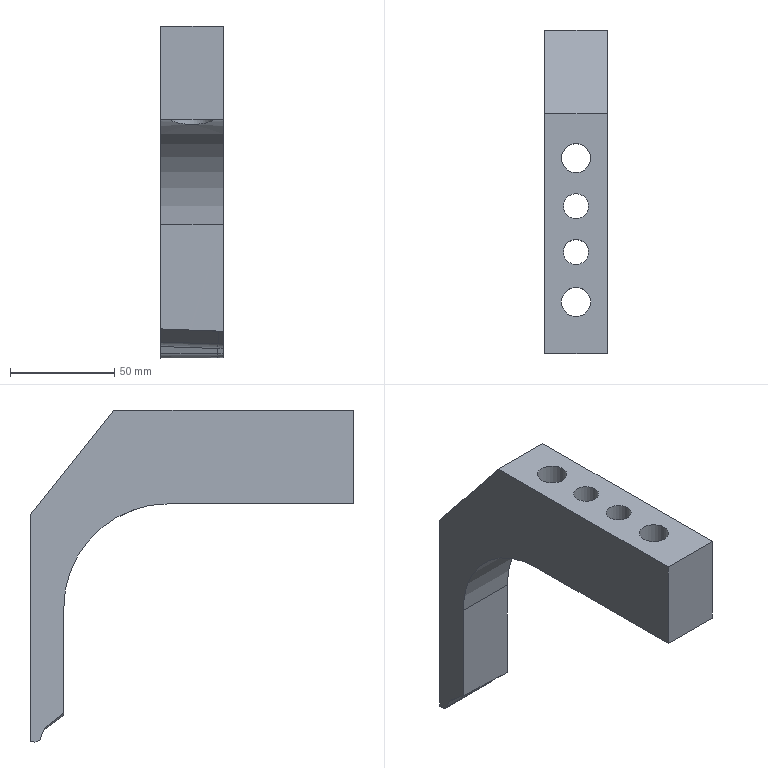Part | NX | features solid 2 | 1 solid | 28 faces | box 30 x 155 x 159.21 mm | volume 216556 mm3 | spline 11 | plane 10 | cylinder 7 | commonest cylinder face diameters 12 x2 14 x2 20 x2 100 x1
STEP:
#1=CARTESIAN_POINT('',(219.476,458.354,-45.808));
#2=VERTEX_POINT('',#1);
#3=CARTESIAN_POINT('',(218.52,458.345,-45.765));
#4=VERTEX_POINT('',#3);
#5=CARTESIAN_POINT('',(219.476,458.35,-45.805));
#6=CARTESIAN_POINT('',(219.157,458.35,-45.791));
#7=CARTESIAN_POINT('',(218.838,458.35,-45.776));
#8=CARTESIAN_POINT('',(218.52,458.35,-45.762));
#9=B_SPLINE_CURVE_WITH_KNOTS('',3,(#5,#6,#7,#8),.UNSPECIFIED.,.F.,.F.,(4,4),(0.,1.),.UNSPECIFIED.);
#10=EDGE_CURVE('',#2,#4,#9,.T.);
#11=ORIENTED_EDGE('',*,*,#10,.F.);
#12=CARTESIAN_POINT('',(235.,458.35,-46.398));
#13=VERTEX_POINT('',#12);
#14=CARTESIAN_POINT('',(219.476,458.35,-45.805));
#15=CARTESIAN_POINT('',(224.651,458.35,-46.003));
#16=CARTESIAN_POINT('',(229.825,458.35,-46.201));
#17=CARTESIAN_POINT('',(235.,458.35,-46.398));
#18=B_SPLINE_CURVE_WITH_KNOTS('',3,(#14,#15,#16,#17),.UNSPECIFIED.,.F.,.F.,(4,4),(0.,0.01554),.UNSPECIFIED.);
#19=EDGE_CURVE('',#2,#13,#18,.T.);
#20=ORIENTED_EDGE('',*,*,#19,.T.);
#21=CARTESIAN_POINT('',(235.,458.35,5.));
#22=VERTEX_POINT('',#21);
#23=CARTESIAN_POINT('',(235.,458.35,-200.));
#24=DIRECTION('',(0.,0.,1.));
#25=VECTOR('',#24,1000.);
#26=LINE('',#23,#25);
#27=EDGE_CURVE('',#13,#22,#26,.T.);
#28=ORIENTED_EDGE('',*,*,#27,.T.);
#29=CARTESIAN_POINT('',(205.,458.35,5.));
#30=VERTEX_POINT('',#29);
#31=CARTESIAN_POINT('',(205.,458.35,5.));
#32=DIRECTION('',(1.,0.,0.));
#33=VECTOR('',#32,1000.);
#34=LINE('',#31,#33);
#35=EDGE_CURVE('',#22,#30,#34,.F.);
#36=ORIENTED_EDGE('',*,*,#35,.T.);
#37=CARTESIAN_POINT('',(205.,458.35,-45.251));
#38=VERTEX_POINT('',#37);
#39=CARTESIAN_POINT('',(205.,458.35,-200.));
#40=DIRECTION('',(0.,0.,1.));
#41=VECTOR('',#40,1000.);
#42=LINE('',#39,#41);
#43=EDGE_CURVE('',#38,#30,#42,.T.);
#44=ORIENTED_EDGE('',*,*,#43,.F.);
#45=CARTESIAN_POINT('',(218.519,458.35,-45.768));
#46=CARTESIAN_POINT('',(214.013,458.35,-45.596));
#47=CARTESIAN_POINT('',(209.506,458.35,-45.423));
#48=CARTESIAN_POINT('',(205.,458.35,-45.251));
#49=B_SPLINE_CURVE_WITH_KNOTS('',3,(#45,#46,#47,#48),.UNSPECIFIED.,.F.,.F.,(4,4),(0.01485,0.02838),.UNSPECIFIED.);
#50=EDGE_CURVE('',#4,#38,#49,.T.);
#51=ORIENTED_EDGE('',*,*,#50,.F.);
#52=EDGE_LOOP('',(#11,#20,#28,#36,#44,#51));
#53=FACE_BOUND('',#52,.T.);
#54=CARTESIAN_POINT('',(220.,458.35,77.5));
#55=DIRECTION('',(0.,1.,0.));
#56=DIRECTION('',(0.,0.,1.));
#57=AXIS2_PLACEMENT_3D('',#54,#55,#56);
#58=PLANE('',#57);
#59=ADVANCED_FACE('',(#53),#58,.F.);
#60=CARTESIAN_POINT('',(235.,474.35,-58.987));
#61=VERTEX_POINT('',#60);
#62=CARTESIAN_POINT('',(235.,472.243,-59.028));
#63=VERTEX_POINT('',#62);
#64=CARTESIAN_POINT('',(235.,474.35,-58.987));
#65=CARTESIAN_POINT('',(235.,473.648,-59.));
#66=CARTESIAN_POINT('',(235.,472.945,-59.014));
#67=CARTESIAN_POINT('',(235.,472.243,-59.028));
#68=B_SPLINE_CURVE_WITH_KNOTS('',3,(#64,#65,#66,#67),.UNSPECIFIED.,.F.,.F.,(4,4),(0.,0.002107),.UNSPECIFIED.);
#69=EDGE_CURVE('',#61,#63,#68,.T.);
#70=ORIENTED_EDGE('',*,*,#69,.F.);
#71=CARTESIAN_POINT('',(235.,474.35,50.));
#72=VERTEX_POINT('',#71);
#73=CARTESIAN_POINT('',(235.,474.35,-200.));
#74=DIRECTION('',(0.,0.,-1.));
#75=VECTOR('',#74,1000.);
#76=LINE('',#73,#75);
#77=EDGE_CURVE('',#72,#61,#76,.T.);
#78=ORIENTED_EDGE('',*,*,#77,.F.);
#79=CARTESIAN_POINT('',(235.,434.35,100.));
#80=VERTEX_POINT('',#79);
#81=CARTESIAN_POINT('',(235.,548.165,-42.268));
#82=DIRECTION('',(0.,0.6247,-0.7809));
#83=VECTOR('',#82,1000.);
#84=LINE('',#81,#83);
#85=EDGE_CURVE('',#72,#80,#84,.F.);
#86=ORIENTED_EDGE('',*,*,#85,.T.);
#87=CARTESIAN_POINT('',(235.,319.35,100.));
#88=VERTEX_POINT('',#87);
#89=CARTESIAN_POINT('',(235.,351.,100.));
#90=DIRECTION('',(0.,1.,0.));
#91=VECTOR('',#90,1000.);
#92=LINE('',#89,#91);
#93=EDGE_CURVE('',#88,#80,#92,.T.);
#94=ORIENTED_EDGE('',*,*,#93,.F.);
#95=CARTESIAN_POINT('',(235.,319.35,55.));
#96=VERTEX_POINT('',#95);
#97=CARTESIAN_POINT('',(235.,319.35,-200.));
#98=DIRECTION('',(0.,0.,1.));
#99=VECTOR('',#98,1000.);
#100=LINE('',#97,#99);
#101=EDGE_CURVE('',#96,#88,#100,.T.);
#102=ORIENTED_EDGE('',*,*,#101,.F.);
#103=CARTESIAN_POINT('',(235.,408.35,55.));
#104=VERTEX_POINT('',#103);
#105=CARTESIAN_POINT('',(235.,351.,55.));
#106=DIRECTION('',(0.,1.,0.));
#107=VECTOR('',#106,1000.);
#108=LINE('',#105,#107);
#109=EDGE_CURVE('',#96,#104,#108,.T.);
#110=ORIENTED_EDGE('',*,*,#109,.T.);
#111=CARTESIAN_POINT('',(235.,408.35,5.));
#112=DIRECTION('',(1.,0.,0.));
#113=DIRECTION('',(0.,0.,-1.));
#114=AXIS2_PLACEMENT_3D('',#111,#112,#113);
#115=CIRCLE('',#114,50.);
#116=EDGE_CURVE('',#104,#22,#115,.F.);
#117=ORIENTED_EDGE('',*,*,#116,.T.);
#118=ORIENTED_EDGE('',*,*,#27,.F.);
#119=CARTESIAN_POINT('',(235.,458.502,-46.511));
#120=VERTEX_POINT('',#119);
#121=CARTESIAN_POINT('',(235.,458.502,-46.511));
#122=CARTESIAN_POINT('',(235.,458.451,-46.474));
#123=CARTESIAN_POINT('',(235.,458.4,-46.437));
#124=CARTESIAN_POINT('',(235.,458.35,-46.398));
#125=B_SPLINE_CURVE_WITH_KNOTS('',3,(#121,#122,#123,#124),.UNSPECIFIED.,.F.,.F.,(4,4),(0.,0.0001883),.UNSPECIFIED.);
#126=EDGE_CURVE('',#120,#13,#125,.T.);
#127=ORIENTED_EDGE('',*,*,#126,.F.);
#128=CARTESIAN_POINT('',(235.,466.758,-52.527));
#129=VERTEX_POINT('',#128);
#130=CARTESIAN_POINT('',(235.,458.502,-46.512));
#131=CARTESIAN_POINT('',(235.,461.253,-48.519));
#132=CARTESIAN_POINT('',(235.,464.006,-50.524));
#133=CARTESIAN_POINT('',(235.,466.76,-52.528));
#134=B_SPLINE_CURVE_WITH_KNOTS('',3,(#130,#131,#132,#133),.UNSPECIFIED.,.F.,.F.,(4,4),(0.00008632,0.0103),.UNSPECIFIED.);
#135=EDGE_CURVE('',#120,#129,#134,.T.);
#136=ORIENTED_EDGE('',*,*,#135,.T.);
#137=CARTESIAN_POINT('',(235.,468.481,-54.772));
#138=VERTEX_POINT('',#137);
#139=CARTESIAN_POINT('',(235.,468.482,-54.771));
#140=CARTESIAN_POINT('',(235.,468.136,-53.875));
#141=CARTESIAN_POINT('',(235.,467.534,-53.091));
#142=CARTESIAN_POINT('',(235.,466.757,-52.526));
#143=B_SPLINE_CURVE_WITH_KNOTS('',3,(#139,#140,#141,#142),.UNSPECIFIED.,.F.,.F.,(4,4),(0.,0.002874),.UNSPECIFIED.);
#144=EDGE_CURVE('',#138,#129,#143,.T.);
#145=ORIENTED_EDGE('',*,*,#144,.F.);
#146=CARTESIAN_POINT('',(235.,469.383,-57.108));
#147=VERTEX_POINT('',#146);
#148=CARTESIAN_POINT('',(235.,469.381,-57.106));
#149=CARTESIAN_POINT('',(235.,469.08,-56.328));
#150=CARTESIAN_POINT('',(235.,468.78,-55.551));
#151=CARTESIAN_POINT('',(235.,468.48,-54.774));
#152=B_SPLINE_CURVE_WITH_KNOTS('',3,(#148,#149,#150,#151),.UNSPECIFIED.,.F.,.F.,(4,4),(0.00004866,0.002549),.UNSPECIFIED.);
#153=EDGE_CURVE('',#147,#138,#152,.T.);
#154=ORIENTED_EDGE('',*,*,#153,.F.);
#155=CARTESIAN_POINT('',(235.,472.243,-59.028));
#156=CARTESIAN_POINT('',(235.,471.011,-59.052));
#157=CARTESIAN_POINT('',(235.,469.83,-58.259));
#158=CARTESIAN_POINT('',(235.,469.386,-57.11));
#159=B_SPLINE_CURVE_WITH_KNOTS('',3,(#155,#156,#157,#158),.UNSPECIFIED.,.F.,.F.,(4,4),(0.,0.003644),.UNSPECIFIED.);
#160=EDGE_CURVE('',#63,#147,#159,.T.);
#161=ORIENTED_EDGE('',*,*,#160,.F.);
#162=EDGE_LOOP('',(#70,#78,#86,#94,#102,#110,#117,#118,#127,#136,#145,#154,#161));
#163=FACE_BOUND('',#162,.T.);
#164=CARTESIAN_POINT('',(235.,351.,-200.));
#165=DIRECTION('',(1.,0.,0.));
#166=DIRECTION('',(0.,0.,-1.));
#167=AXIS2_PLACEMENT_3D('',#164,#165,#166);
#168=PLANE('',#167);
#169=ADVANCED_FACE('',(#163),#168,.T.);
#170=CARTESIAN_POINT('',(205.,474.35,50.));
#171=VERTEX_POINT('',#170);
#172=CARTESIAN_POINT('',(205.,474.35,-59.17));
#173=VERTEX_POINT('',#172);
#174=CARTESIAN_POINT('',(205.,474.35,-200.));
#175=DIRECTION('',(0.,0.,-1.));
#176=VECTOR('',#175,1000.);
#177=LINE('',#174,#176);
#178=EDGE_CURVE('',#171,#173,#177,.T.);
#179=ORIENTED_EDGE('',*,*,#178,.T.);
#180=CARTESIAN_POINT('',(205.,472.244,-59.21));
#181=VERTEX_POINT('',#180);
#182=CARTESIAN_POINT('',(205.,474.35,-59.17));
#183=CARTESIAN_POINT('',(205.,473.646,-59.183));
#184=CARTESIAN_POINT('',(205.,472.942,-59.197));
#185=CARTESIAN_POINT('',(205.,472.239,-59.21));
#186=B_SPLINE_CURVE_WITH_KNOTS('',3,(#182,#183,#184,#185),.UNSPECIFIED.,.F.,.F.,(4,4),(0.,0.002112),.UNSPECIFIED.);
#187=EDGE_CURVE('',#173,#181,#186,.T.);
#188=ORIENTED_EDGE('',*,*,#187,.T.);
#189=CARTESIAN_POINT('',(205.,469.389,-57.288));
#190=VERTEX_POINT('',#189);
#191=CARTESIAN_POINT('',(205.,472.245,-59.21));
#192=CARTESIAN_POINT('',(205.,471.012,-59.232));
#193=CARTESIAN_POINT('',(205.,469.832,-58.438));
#194=CARTESIAN_POINT('',(205.,469.389,-57.288));
#195=B_SPLINE_CURVE_WITH_KNOTS('',3,(#191,#192,#193,#194),.UNSPECIFIED.,.F.,.F.,(4,4),(0.,0.003644),.UNSPECIFIED.);
#196=EDGE_CURVE('',#181,#190,#195,.T.);
#197=ORIENTED_EDGE('',*,*,#196,.T.);
#198=CARTESIAN_POINT('',(205.,468.012,-53.711));
#199=VERTEX_POINT('',#198);
#200=CARTESIAN_POINT('',(205.,469.389,-57.288));
#201=CARTESIAN_POINT('',(205.,468.93,-56.096));
#202=CARTESIAN_POINT('',(205.,468.471,-54.903));
#203=CARTESIAN_POINT('',(205.,468.012,-53.711));
#204=B_SPLINE_CURVE_WITH_KNOTS('',3,(#200,#201,#202,#203),.UNSPECIFIED.,.F.,.F.,(4,4),(0.0000259,0.003859),.UNSPECIFIED.);
#205=EDGE_CURVE('',#190,#199,#204,.T.);
#206=ORIENTED_EDGE('',*,*,#205,.T.);
#207=CARTESIAN_POINT('',(205.,466.425,-51.567));
#208=VERTEX_POINT('',#207);
#209=CARTESIAN_POINT('',(205.,468.012,-53.711));
#210=CARTESIAN_POINT('',(205.,467.688,-52.868));
#211=CARTESIAN_POINT('',(205.,467.136,-52.123));
#212=CARTESIAN_POINT('',(205.,466.425,-51.567));
#213=B_SPLINE_CURVE_WITH_KNOTS('',3,(#209,#210,#211,#212),.UNSPECIFIED.,.F.,.F.,(4,4),(0.,0.002703),.UNSPECIFIED.);
#214=EDGE_CURVE('',#199,#208,#213,.T.);
#215=ORIENTED_EDGE('',*,*,#214,.T.);
#216=CARTESIAN_POINT('',(205.,458.35,-45.251));
#217=CARTESIAN_POINT('',(205.,461.041,-47.356));
#218=CARTESIAN_POINT('',(205.,463.733,-49.461));
#219=CARTESIAN_POINT('',(205.,466.425,-51.567));
#220=B_SPLINE_CURVE_WITH_KNOTS('',3,(#216,#217,#218,#219),.UNSPECIFIED.,.F.,.F.,(4,4),(0.0006093,0.01086),.UNSPECIFIED.);
#221=EDGE_CURVE('',#38,#208,#220,.T.);
#222=ORIENTED_EDGE('',*,*,#221,.F.);
#223=ORIENTED_EDGE('',*,*,#43,.T.);
#224=CARTESIAN_POINT('',(205.,408.35,55.));
#225=VERTEX_POINT('',#224);
#226=CARTESIAN_POINT('',(205.,408.35,5.));
#227=DIRECTION('',(1.,0.,0.));
#228=DIRECTION('',(0.,0.,-1.));
#229=AXIS2_PLACEMENT_3D('',#226,#227,#228);
#230=CIRCLE('',#229,50.);
#231=EDGE_CURVE('',#30,#225,#230,.T.);
#232=ORIENTED_EDGE('',*,*,#231,.T.);
#233=CARTESIAN_POINT('',(205.,319.35,55.));
#234=VERTEX_POINT('',#233);
#235=CARTESIAN_POINT('',(205.,431.,55.));
#236=DIRECTION('',(0.,1.,0.));
#237=VECTOR('',#236,1000.);
#238=LINE('',#235,#237);
#239=EDGE_CURVE('',#225,#234,#238,.F.);
#240=ORIENTED_EDGE('',*,*,#239,.T.);
#241=CARTESIAN_POINT('',(205.,319.35,100.));
#242=VERTEX_POINT('',#241);
#243=CARTESIAN_POINT('',(205.,319.35,-200.));
#244=DIRECTION('',(0.,0.,1.));
#245=VECTOR('',#244,1000.);
#246=LINE('',#243,#245);
#247=EDGE_CURVE('',#234,#242,#246,.T.);
#248=ORIENTED_EDGE('',*,*,#247,.T.);
#249=CARTESIAN_POINT('',(205.,434.35,100.));
#250=VERTEX_POINT('',#249);
#251=CARTESIAN_POINT('',(205.,351.,100.));
#252=DIRECTION('',(0.,1.,0.));
#253=VECTOR('',#252,1000.);
#254=LINE('',#251,#253);
#255=EDGE_CURVE('',#242,#250,#254,.T.);
#256=ORIENTED_EDGE('',*,*,#255,.T.);
#257=CARTESIAN_POINT('',(205.,434.35,100.));
#258=DIRECTION('',(0.,-0.6247,0.7809));
#259=VECTOR('',#258,1000.);
#260=LINE('',#257,#259);
#261=EDGE_CURVE('',#250,#171,#260,.F.);
#262=ORIENTED_EDGE('',*,*,#261,.T.);
#263=EDGE_LOOP('',(#179,#188,#197,#206,#215,#222,#223,#232,#240,#248,#256,#262));
#264=FACE_BOUND('',#263,.T.);
#265=CARTESIAN_POINT('',(205.,351.,-200.));
#266=DIRECTION('',(1.,0.,0.));
#267=DIRECTION('',(0.,0.,-1.));
#268=AXIS2_PLACEMENT_3D('',#265,#266,#267);
#269=PLANE('',#268);
#270=ADVANCED_FACE('',(#264),#269,.F.);
#271=ORIENTED_EDGE('',*,*,#247,.F.);
#272=CARTESIAN_POINT('',(235.,319.35,55.));
#273=DIRECTION('',(-1.,0.,0.));
#274=VECTOR('',#273,1000.);
#275=LINE('',#272,#274);
#276=EDGE_CURVE('',#96,#234,#275,.T.);
#277=ORIENTED_EDGE('',*,*,#276,.F.);
#278=ORIENTED_EDGE('',*,*,#101,.T.);
#279=CARTESIAN_POINT('',(275.,319.35,100.));
#280=DIRECTION('',(-1.,0.,0.));
#281=VECTOR('',#280,1000.);
#282=LINE('',#279,#281);
#283=EDGE_CURVE('',#88,#242,#282,.T.);
#284=ORIENTED_EDGE('',*,*,#283,.T.);
#285=EDGE_LOOP('',(#271,#277,#278,#284));
#286=FACE_BOUND('',#285,.T.);
#287=CARTESIAN_POINT('',(275.,319.35,75.));
#288=DIRECTION('',(0.,1.,0.));
#289=DIRECTION('',(0.,0.,1.));
#290=AXIS2_PLACEMENT_3D('',#287,#288,#289);
#291=PLANE('',#290);
#292=ADVANCED_FACE('',(#286),#291,.F.);
#293=CARTESIAN_POINT('',(214.,368.,100.));
#294=VERTEX_POINT('',#293);
#295=CARTESIAN_POINT('',(220.,368.,100.));
#296=DIRECTION('',(0.,0.,-1.));
#297=DIRECTION('',(-1.,0.,0.));
#298=AXIS2_PLACEMENT_3D('',#295,#296,#297);
#299=CIRCLE('',#298,6.);
#300=EDGE_CURVE('',#294,#294,#299,.T.);
#301=ORIENTED_EDGE('',*,*,#300,.T.);
#302=EDGE_LOOP('',(#301));
#303=FACE_BOUND('',#302,.T.);
#304=CARTESIAN_POINT('',(214.,390.,100.));
#305=VERTEX_POINT('',#304);
#306=CARTESIAN_POINT('',(220.,390.,100.));
#307=DIRECTION('',(0.,0.,-1.));
#308=DIRECTION('',(-1.,0.,0.));
#309=AXIS2_PLACEMENT_3D('',#306,#307,#308);
#310=CIRCLE('',#309,6.);
#311=EDGE_CURVE('',#305,#305,#310,.T.);
#312=ORIENTED_EDGE('',*,*,#311,.T.);
#313=EDGE_LOOP('',(#312));
#314=FACE_BOUND('',#313,.T.);
#315=CARTESIAN_POINT('',(213.,344.,100.));
#316=VERTEX_POINT('',#315);
#317=CARTESIAN_POINT('',(220.,344.,100.));
#318=DIRECTION('',(0.,0.,-1.));
#319=DIRECTION('',(-1.,0.,0.));
#320=AXIS2_PLACEMENT_3D('',#317,#318,#319);
#321=CIRCLE('',#320,7.);
#322=EDGE_CURVE('',#316,#316,#321,.T.);
#323=ORIENTED_EDGE('',*,*,#322,.T.);
#324=EDGE_LOOP('',(#323));
#325=FACE_BOUND('',#324,.T.);
#326=CARTESIAN_POINT('',(213.,413.,100.));
#327=VERTEX_POINT('',#326);
#328=CARTESIAN_POINT('',(220.,413.,100.));
#329=DIRECTION('',(0.,0.,-1.));
#330=DIRECTION('',(-1.,0.,0.));
#331=AXIS2_PLACEMENT_3D('',#328,#329,#330);
#332=CIRCLE('',#331,7.);
#333=EDGE_CURVE('',#327,#327,#332,.T.);
#334=ORIENTED_EDGE('',*,*,#333,.T.);
#335=EDGE_LOOP('',(#334));
#336=FACE_BOUND('',#335,.T.);
#337=ORIENTED_EDGE('',*,*,#93,.T.);
#338=CARTESIAN_POINT('',(160.,434.35,100.));
#339=DIRECTION('',(-1.,0.,0.));
#340=VECTOR('',#339,1000.);
#341=LINE('',#338,#340);
#342=EDGE_CURVE('',#80,#250,#341,.T.);
#343=ORIENTED_EDGE('',*,*,#342,.T.);
#344=ORIENTED_EDGE('',*,*,#255,.F.);
#345=ORIENTED_EDGE('',*,*,#283,.F.);
#346=EDGE_LOOP('',(#337,#343,#344,#345));
#347=FACE_BOUND('',#346,.T.);
#348=CARTESIAN_POINT('',(160.,351.,100.));
#349=DIRECTION('',(0.,0.,-1.));
#350=DIRECTION('',(-1.,0.,0.));
#351=AXIS2_PLACEMENT_3D('',#348,#349,#350);
#352=PLANE('',#351);
#353=ADVANCED_FACE('',(#303,#314,#325,#336,#347),#352,.F.);
#354=CARTESIAN_POINT('',(227.,413.,75.));
#355=VERTEX_POINT('',#354);
#356=CARTESIAN_POINT('',(220.,413.,75.));
#357=DIRECTION('',(0.,0.,1.));
#358=DIRECTION('',(1.,0.,0.));
#359=AXIS2_PLACEMENT_3D('',#356,#357,#358);
#360=CIRCLE('',#359,7.);
#361=EDGE_CURVE('',#355,#355,#360,.T.);
#362=ORIENTED_EDGE('',*,*,#361,.F.);
#363=EDGE_LOOP('',(#362));
#364=FACE_BOUND('',#363,.T.);
#365=ORIENTED_EDGE('',*,*,#333,.F.);
#366=EDGE_LOOP('',(#365));
#367=FACE_BOUND('',#366,.T.);
#368=CARTESIAN_POINT('',(220.,413.,75.));
#369=DIRECTION('',(0.,0.,1.));
#370=DIRECTION('',(-1.,0.,0.));
#371=AXIS2_PLACEMENT_3D('',#368,#369,#370);
#372=CYLINDRICAL_SURFACE('',#371,7.);
#373=ADVANCED_FACE('',(#364,#367),#372,.F.);
#374=ORIENTED_EDGE('',*,*,#361,.T.);
#375=EDGE_LOOP('',(#374));
#376=FACE_BOUND('',#375,.T.);
#377=CARTESIAN_POINT('',(230.,413.,75.));
#378=VERTEX_POINT('',#377);
#379=CARTESIAN_POINT('',(220.,413.,75.));
#380=DIRECTION('',(0.,0.,-1.));
#381=DIRECTION('',(1.,0.,0.));
#382=AXIS2_PLACEMENT_3D('',#379,#380,#381);
#383=CIRCLE('',#382,10.);
#384=EDGE_CURVE('',#378,#378,#383,.T.);
#385=ORIENTED_EDGE('',*,*,#384,.T.);
#386=EDGE_LOOP('',(#385));
#387=FACE_BOUND('',#386,.T.);
#388=CARTESIAN_POINT('',(220.,413.,75.));
#389=DIRECTION('',(0.,0.,1.));
#390=DIRECTION('',(-1.,0.,0.));
#391=AXIS2_PLACEMENT_3D('',#388,#389,#390);
#392=PLANE('',#391);
#393=ADVANCED_FACE('',(#376,#387),#392,.F.);
#394=CARTESIAN_POINT('',(228.853,408.35,55.));
#395=VERTEX_POINT('',#394);
#396=CARTESIAN_POINT('',(211.147,408.35,55.));
#397=VERTEX_POINT('',#396);
#398=CARTESIAN_POINT('',(220.,413.,55.));
#399=DIRECTION('',(0.,0.,1.));
#400=DIRECTION('',(1.,0.,0.));
#401=AXIS2_PLACEMENT_3D('',#398,#399,#400);
#402=CIRCLE('',#401,10.);
#403=EDGE_CURVE('',#395,#397,#402,.F.);
#404=ORIENTED_EDGE('',*,*,#403,.T.);
#405=CARTESIAN_POINT('',(211.147,408.35,55.));
#406=CARTESIAN_POINT('',(210.338,409.891,55.));
#407=CARTESIAN_POINT('',(209.557,413.344,54.846));
#408=CARTESIAN_POINT('',(211.077,418.422,54.048));
#409=CARTESIAN_POINT('',(214.831,422.077,53.101));
#410=CARTESIAN_POINT('',(219.999,423.459,52.658));
#411=CARTESIAN_POINT('',(225.153,422.088,53.099));
#412=CARTESIAN_POINT('',(228.929,418.412,54.049));
#413=CARTESIAN_POINT('',(230.441,413.366,54.844));
#414=CARTESIAN_POINT('',(229.663,409.891,55.));
#415=CARTESIAN_POINT('',(228.853,408.35,55.));
#416=B_SPLINE_CURVE_WITH_KNOTS('',3,(#405,#406,#407,#408,#409,#410,#411,#412,#413,#414,#415),.UNSPECIFIED.,.F.,.F.,(4,1,1,1,1,1,1,1,4),(0.,0.005148,0.0103,0.01544,0.02059,0.02574,0.03089,0.03603,0.04118),.UNSPECIFIED.);
#417=EDGE_CURVE('',#397,#395,#416,.T.);
#418=ORIENTED_EDGE('',*,*,#417,.T.);
#419=EDGE_LOOP('',(#404,#418));
#420=FACE_BOUND('',#419,.T.);
#421=ORIENTED_EDGE('',*,*,#384,.F.);
#422=EDGE_LOOP('',(#421));
#423=FACE_BOUND('',#422,.T.);
#424=CARTESIAN_POINT('',(220.,413.,75.));
#425=DIRECTION('',(0.,0.,-1.));
#426=DIRECTION('',(1.,0.,0.));
#427=AXIS2_PLACEMENT_3D('',#424,#425,#426);
#428=CYLINDRICAL_SURFACE('',#427,10.);
#429=ADVANCED_FACE('',(#420,#423),#428,.F.);
#430=CARTESIAN_POINT('',(227.,344.,75.));
#431=VERTEX_POINT('',#430);
#432=CARTESIAN_POINT('',(220.,344.,75.));
#433=DIRECTION('',(0.,0.,1.));
#434=DIRECTION('',(1.,0.,0.));
#435=AXIS2_PLACEMENT_3D('',#432,#433,#434);
#436=CIRCLE('',#435,7.);
#437=EDGE_CURVE('',#431,#431,#436,.T.);
#438=ORIENTED_EDGE('',*,*,#437,.F.);
#439=EDGE_LOOP('',(#438));
#440=FACE_BOUND('',#439,.T.);
#441=ORIENTED_EDGE('',*,*,#322,.F.);
#442=EDGE_LOOP('',(#441));
#443=FACE_BOUND('',#442,.T.);
#444=CARTESIAN_POINT('',(220.,344.,75.));
#445=DIRECTION('',(0.,0.,1.));
#446=DIRECTION('',(-1.,0.,0.));
#447=AXIS2_PLACEMENT_3D('',#444,#445,#446);
#448=CYLINDRICAL_SURFACE('',#447,7.);
#449=ADVANCED_FACE('',(#440,#443),#448,.F.);
#450=CARTESIAN_POINT('',(230.,344.,55.));
#451=VERTEX_POINT('',#450);
#452=CARTESIAN_POINT('',(220.,344.,55.));
#453=DIRECTION('',(0.,0.,1.));
#454=DIRECTION('',(1.,0.,0.));
#455=AXIS2_PLACEMENT_3D('',#452,#453,#454);
#456=CIRCLE('',#455,10.);
#457=EDGE_CURVE('',#451,#451,#456,.F.);
#458=ORIENTED_EDGE('',*,*,#457,.T.);
#459=EDGE_LOOP('',(#458));
#460=FACE_BOUND('',#459,.T.);
#461=CARTESIAN_POINT('',(230.,344.,75.));
#462=VERTEX_POINT('',#461);
#463=CARTESIAN_POINT('',(220.,344.,75.));
#464=DIRECTION('',(0.,0.,-1.));
#465=DIRECTION('',(1.,0.,0.));
#466=AXIS2_PLACEMENT_3D('',#463,#464,#465);
#467=CIRCLE('',#466,10.);
#468=EDGE_CURVE('',#462,#462,#467,.T.);
#469=ORIENTED_EDGE('',*,*,#468,.F.);
#470=EDGE_LOOP('',(#469));
#471=FACE_BOUND('',#470,.T.);
#472=CARTESIAN_POINT('',(220.,344.,75.));
#473=DIRECTION('',(0.,0.,-1.));
#474=DIRECTION('',(1.,0.,0.));
#475=AXIS2_PLACEMENT_3D('',#472,#473,#474);
#476=CYLINDRICAL_SURFACE('',#475,10.);
#477=ADVANCED_FACE('',(#460,#471),#476,.F.);
#478=ORIENTED_EDGE('',*,*,#437,.T.);
#479=EDGE_LOOP('',(#478));
#480=FACE_BOUND('',#479,.T.);
#481=ORIENTED_EDGE('',*,*,#468,.T.);
#482=EDGE_LOOP('',(#481));
#483=FACE_BOUND('',#482,.T.);
#484=CARTESIAN_POINT('',(220.,344.,75.));
#485=DIRECTION('',(0.,0.,1.));
#486=DIRECTION('',(-1.,0.,0.));
#487=AXIS2_PLACEMENT_3D('',#484,#485,#486);
#488=PLANE('',#487);
#489=ADVANCED_FACE('',(#480,#483),#488,.F.);
#490=CARTESIAN_POINT('',(214.,368.,55.));
#491=VERTEX_POINT('',#490);
#492=CARTESIAN_POINT('',(220.,368.,55.));
#493=DIRECTION('',(0.,0.,-1.));
#494=DIRECTION('',(-1.,0.,0.));
#495=AXIS2_PLACEMENT_3D('',#492,#493,#494);
#496=CIRCLE('',#495,6.);
#497=EDGE_CURVE('',#491,#491,#496,.T.);
#498=ORIENTED_EDGE('',*,*,#497,.F.);
#499=EDGE_LOOP('',(#498));
#500=FACE_BOUND('',#499,.T.);
#501=CARTESIAN_POINT('',(214.,390.,55.));
#502=VERTEX_POINT('',#501);
#503=CARTESIAN_POINT('',(220.,390.,55.));
#504=DIRECTION('',(0.,0.,-1.));
#505=DIRECTION('',(-1.,0.,0.));
#506=AXIS2_PLACEMENT_3D('',#503,#504,#505);
#507=CIRCLE('',#506,6.);
#508=EDGE_CURVE('',#502,#502,#507,.T.);
#509=ORIENTED_EDGE('',*,*,#508,.F.);
#510=EDGE_LOOP('',(#509));
#511=FACE_BOUND('',#510,.T.);
#512=ORIENTED_EDGE('',*,*,#457,.F.);
#513=EDGE_LOOP('',(#512));
#514=FACE_BOUND('',#513,.T.);
#515=ORIENTED_EDGE('',*,*,#239,.F.);
#516=CARTESIAN_POINT('',(235.,408.35,55.));
#517=DIRECTION('',(1.,0.,0.));
#518=VECTOR('',#517,1000.);
#519=LINE('',#516,#518);
#520=EDGE_CURVE('',#225,#397,#519,.T.);
#521=ORIENTED_EDGE('',*,*,#520,.T.);
#522=ORIENTED_EDGE('',*,*,#403,.F.);
#523=CARTESIAN_POINT('',(235.,408.35,55.));
#524=DIRECTION('',(1.,0.,0.));
#525=VECTOR('',#524,1000.);
#526=LINE('',#523,#525);
#527=EDGE_CURVE('',#395,#104,#526,.T.);
#528=ORIENTED_EDGE('',*,*,#527,.T.);
#529=ORIENTED_EDGE('',*,*,#109,.F.);
#530=ORIENTED_EDGE('',*,*,#276,.T.);
#531=EDGE_LOOP('',(#515,#521,#522,#528,#529,#530));
#532=FACE_BOUND('',#531,.T.);
#533=CARTESIAN_POINT('',(235.,431.,55.));
#534=DIRECTION('',(0.,0.,1.));
#535=DIRECTION('',(1.,0.,0.));
#536=AXIS2_PLACEMENT_3D('',#533,#534,#535);
#537=PLANE('',#536);
#538=ADVANCED_FACE('',(#500,#511,#514,#532),#537,.F.);
#539=ORIENTED_EDGE('',*,*,#311,.F.);
#540=EDGE_LOOP('',(#539));
#541=FACE_BOUND('',#540,.T.);
#542=ORIENTED_EDGE('',*,*,#508,.T.);
#543=EDGE_LOOP('',(#542));
#544=FACE_BOUND('',#543,.T.);
#545=CARTESIAN_POINT('',(220.,390.,105.));
#546=DIRECTION('',(0.,0.,-1.));
#547=DIRECTION('',(-1.,0.,0.));
#548=AXIS2_PLACEMENT_3D('',#545,#546,#547);
#549=CYLINDRICAL_SURFACE('',#548,6.);
#550=ADVANCED_FACE('',(#541,#544),#549,.F.);
#551=ORIENTED_EDGE('',*,*,#300,.F.);
#552=EDGE_LOOP('',(#551));
#553=FACE_BOUND('',#552,.T.);
#554=ORIENTED_EDGE('',*,*,#497,.T.);
#555=EDGE_LOOP('',(#554));
#556=FACE_BOUND('',#555,.T.);
#557=CARTESIAN_POINT('',(220.,368.,105.));
#558=DIRECTION('',(0.,0.,-1.));
#559=DIRECTION('',(-1.,0.,0.));
#560=AXIS2_PLACEMENT_3D('',#557,#558,#559);
#561=CYLINDRICAL_SURFACE('',#560,6.);
#562=ADVANCED_FACE('',(#553,#556),#561,.F.);
#563=ORIENTED_EDGE('',*,*,#77,.T.);
#564=CARTESIAN_POINT('',(232.114,474.35,-59.018));
#565=VERTEX_POINT('',#564);
#566=CARTESIAN_POINT('',(235.,474.35,-58.987));
#567=CARTESIAN_POINT('',(234.038,474.35,-58.997));
#568=CARTESIAN_POINT('',(233.076,474.35,-59.008));
#569=CARTESIAN_POINT('',(232.114,474.35,-59.018));
#570=B_SPLINE_CURVE_WITH_KNOTS('',3,(#566,#567,#568,#569),.UNSPECIFIED.,.F.,.F.,(4,4),(0.,0.002886),.UNSPECIFIED.);
#571=EDGE_CURVE('',#61,#565,#570,.T.);
#572=ORIENTED_EDGE('',*,*,#571,.T.);
#573=CARTESIAN_POINT('',(232.114,474.35,-59.018));
#574=CARTESIAN_POINT('',(223.076,474.35,-59.111));
#575=CARTESIAN_POINT('',(214.038,474.35,-59.162));
#576=CARTESIAN_POINT('',(205.,474.35,-59.17));
#577=B_SPLINE_CURVE_WITH_KNOTS('',3,(#573,#574,#575,#576),.UNSPECIFIED.,.F.,.F.,(4,4),(0.00001661,0.02713),.UNSPECIFIED.);
#578=EDGE_CURVE('',#565,#173,#577,.T.);
#579=ORIENTED_EDGE('',*,*,#578,.T.);
#580=ORIENTED_EDGE('',*,*,#178,.F.);
#581=CARTESIAN_POINT('',(220.,474.35,50.));
#582=DIRECTION('',(1.,0.,0.));
#583=VECTOR('',#582,1000.);
#584=LINE('',#581,#583);
#585=EDGE_CURVE('',#171,#72,#584,.T.);
#586=ORIENTED_EDGE('',*,*,#585,.T.);
#587=EDGE_LOOP('',(#563,#572,#579,#580,#586));
#588=FACE_BOUND('',#587,.T.);
#589=CARTESIAN_POINT('',(220.,474.35,77.5));
#590=DIRECTION('',(0.,-1.,0.));
#591=DIRECTION('',(0.,0.,-1.));
#592=AXIS2_PLACEMENT_3D('',#589,#590,#591);
#593=PLANE('',#592);
#594=ADVANCED_FACE('',(#588),#593,.F.);
#595=ORIENTED_EDGE('',*,*,#231,.F.);
#596=ORIENTED_EDGE('',*,*,#35,.F.);
#597=ORIENTED_EDGE('',*,*,#116,.F.);
#598=ORIENTED_EDGE('',*,*,#527,.F.);
#599=ORIENTED_EDGE('',*,*,#417,.F.);
#600=ORIENTED_EDGE('',*,*,#520,.F.);
#601=EDGE_LOOP('',(#595,#596,#597,#598,#599,#600));
#602=FACE_BOUND('',#601,.T.);
#603=CARTESIAN_POINT('',(235.,408.35,5.));
#604=DIRECTION('',(-1.,0.,0.));
#605=DIRECTION('',(0.,0.,1.));
#606=AXIS2_PLACEMENT_3D('',#603,#604,#605);
#607=CYLINDRICAL_SURFACE('',#606,50.);
#608=ADVANCED_FACE('',(#602),#607,.F.);
#609=ORIENTED_EDGE('',*,*,#85,.F.);
#610=ORIENTED_EDGE('',*,*,#585,.F.);
#611=ORIENTED_EDGE('',*,*,#261,.F.);
#612=ORIENTED_EDGE('',*,*,#342,.F.);
#613=EDGE_LOOP('',(#609,#610,#611,#612));
#614=FACE_BOUND('',#613,.T.);
#615=CARTESIAN_POINT('',(160.,434.35,100.));
#616=DIRECTION('',(0.,-0.7809,-0.6247));
#617=DIRECTION('',(0.,0.6247,-0.7809));
#618=AXIS2_PLACEMENT_3D('',#615,#616,#617);
#619=PLANE('',#618);
#620=ADVANCED_FACE('',(#614),#619,.F.);
#621=CARTESIAN_POINT('',(232.133,472.243,-59.059));
#622=VERTEX_POINT('',#621);
#623=CARTESIAN_POINT('',(232.133,472.243,-59.059));
#624=CARTESIAN_POINT('',(223.089,472.244,-59.151));
#625=CARTESIAN_POINT('',(214.045,472.244,-59.202));
#626=CARTESIAN_POINT('',(205.,472.245,-59.21));
#627=B_SPLINE_CURVE_WITH_KNOTS('',3,(#623,#624,#625,#626),.UNSPECIFIED.,.F.,.F.,(4,4),(0.,0.6639),.UNSPECIFIED.);
#628=EDGE_CURVE('',#181,#622,#627,.F.);
#629=ORIENTED_EDGE('',*,*,#628,.T.);
#630=CARTESIAN_POINT('',(232.249,469.383,-57.14));
#631=VERTEX_POINT('',#630);
#632=CARTESIAN_POINT('',(232.249,469.386,-57.139));
#633=CARTESIAN_POINT('',(232.215,469.65,-57.824));
#634=CARTESIAN_POINT('',(232.162,470.634,-58.849));
#635=CARTESIAN_POINT('',(232.137,471.756,-59.068));
#636=CARTESIAN_POINT('',(232.133,472.243,-59.059));
#637=B_SPLINE_CURVE_WITH_KNOTS('',3,(#632,#633,#634,#635,#636),.UNSPECIFIED.,.F.,.F.,(4,1,4),(0.,0.5,1.),.UNSPECIFIED.);
#638=EDGE_CURVE('',#622,#631,#637,.F.);
#639=ORIENTED_EDGE('',*,*,#638,.T.);
#640=CARTESIAN_POINT('',(205.,469.389,-57.288));
#641=CARTESIAN_POINT('',(214.083,469.388,-57.281));
#642=CARTESIAN_POINT('',(223.166,469.387,-57.231));
#643=CARTESIAN_POINT('',(232.249,469.386,-57.139));
#644=B_SPLINE_CURVE_WITH_KNOTS('',3,(#640,#641,#642,#643),.UNSPECIFIED.,.F.,.F.,(4,4),(0.3351,1.),.UNSPECIFIED.);
#645=EDGE_CURVE('',#190,#631,#644,.T.);
#646=ORIENTED_EDGE('',*,*,#645,.F.);
#647=ORIENTED_EDGE('',*,*,#196,.F.);
#648=EDGE_LOOP('',(#629,#639,#646,#647));
#649=FACE_BOUND('',#648,.T.);
#650=CARTESIAN_POINT('',(232.269,472.243,-59.057));
#651=CARTESIAN_POINT('',(232.269,471.51,-59.072));
#652=CARTESIAN_POINT('',(232.266,470.773,-58.862));
#653=CARTESIAN_POINT('',(232.262,470.123,-58.426));
#654=CARTESIAN_POINT('',(232.256,469.65,-57.823));
#655=CARTESIAN_POINT('',(232.249,469.386,-57.139));
#656=CARTESIAN_POINT('',(226.783,472.244,-59.114));
#657=CARTESIAN_POINT('',(226.783,471.511,-59.128));
#658=CARTESIAN_POINT('',(226.781,470.773,-58.918));
#659=CARTESIAN_POINT('',(226.777,470.123,-58.482));
#660=CARTESIAN_POINT('',(226.772,469.651,-57.879));
#661=CARTESIAN_POINT('',(226.766,469.387,-57.195));
#662=CARTESIAN_POINT('',(221.296,472.244,-59.157));
#663=CARTESIAN_POINT('',(221.296,471.511,-59.171));
#664=CARTESIAN_POINT('',(221.295,470.774,-58.961));
#665=CARTESIAN_POINT('',(221.292,470.124,-58.525));
#666=CARTESIAN_POINT('',(221.288,469.651,-57.921));
#667=CARTESIAN_POINT('',(221.283,469.387,-57.237));
#668=CARTESIAN_POINT('',(215.81,472.244,-59.188));
#669=CARTESIAN_POINT('',(215.81,471.511,-59.202));
#670=CARTESIAN_POINT('',(215.809,470.774,-58.992));
#671=CARTESIAN_POINT('',(215.807,470.124,-58.555));
#672=CARTESIAN_POINT('',(215.804,469.652,-57.951));
#673=CARTESIAN_POINT('',(215.8,469.388,-57.267));
#674=CARTESIAN_POINT('',(210.323,472.244,-59.205));
#675=CARTESIAN_POINT('',(210.323,471.511,-59.219));
#676=CARTESIAN_POINT('',(210.322,470.774,-59.009));
#677=CARTESIAN_POINT('',(210.321,470.125,-58.572));
#678=CARTESIAN_POINT('',(210.319,469.652,-57.968));
#679=CARTESIAN_POINT('',(210.317,469.388,-57.284));
#680=CARTESIAN_POINT('',(204.836,472.245,-59.21));
#681=CARTESIAN_POINT('',(204.836,471.512,-59.223));
#682=CARTESIAN_POINT('',(204.836,470.774,-59.013));
#683=CARTESIAN_POINT('',(204.836,470.125,-58.576));
#684=CARTESIAN_POINT('',(204.835,469.653,-57.972));
#685=CARTESIAN_POINT('',(204.834,469.389,-57.288));
#686=B_SPLINE_SURFACE_WITH_KNOTS('',5,5,((#650,#651,#652,#653,#654,#655),(#656,#657,#658,#659,#660,#661),(#662,#663,#664,#665,#666,#667),(#668,#669,#670,#671,#672,#673),(#674,#675,#676,#677,#678,#679),(#680,#681,#682,#683,#684,#685)),.UNSPECIFIED.,.F.,.F.,.F.,(6,6),(6,6),(0.,0.669),(0.,1.),.PIECEWISE_BEZIER_KNOTS.);
#687=ADVANCED_FACE('',(#649),#686,.F.);
#688=ORIENTED_EDGE('',*,*,#645,.T.);
#689=CARTESIAN_POINT('',(232.37,468.432,-54.676));
#690=VERTEX_POINT('',#689);
#691=CARTESIAN_POINT('',(232.37,468.435,-54.675));
#692=CARTESIAN_POINT('',(232.329,468.752,-55.496));
#693=CARTESIAN_POINT('',(232.289,469.069,-56.318));
#694=CARTESIAN_POINT('',(232.249,469.386,-57.139));
#695=B_SPLINE_CURVE_WITH_KNOTS('',3,(#691,#692,#693,#694),.UNSPECIFIED.,.F.,.F.,(4,4),(0.,1.),.UNSPECIFIED.);
#696=EDGE_CURVE('',#631,#690,#695,.F.);
#697=ORIENTED_EDGE('',*,*,#696,.T.);
#698=CARTESIAN_POINT('',(205.,468.012,-53.711));
#699=CARTESIAN_POINT('',(214.001,468.13,-54.018));
#700=CARTESIAN_POINT('',(223.124,468.271,-54.34));
#701=CARTESIAN_POINT('',(232.37,468.435,-54.675));
#702=B_SPLINE_CURVE_WITH_KNOTS('',3,(#698,#699,#700,#701),.UNSPECIFIED.,.F.,.F.,(4,4),(0.3467,1.),.UNSPECIFIED.);
#703=EDGE_CURVE('',#199,#690,#702,.T.);
#704=ORIENTED_EDGE('',*,*,#703,.F.);
#705=ORIENTED_EDGE('',*,*,#205,.F.);
#706=EDGE_LOOP('',(#688,#697,#704,#705));
#707=FACE_BOUND('',#706,.T.);
#708=CARTESIAN_POINT('',(204.833,468.004,-53.69));
#709=CARTESIAN_POINT('',(204.836,469.397,-57.309));
#710=CARTESIAN_POINT('',(210.371,468.002,-53.686));
#711=CARTESIAN_POINT('',(210.381,469.397,-57.306));
#712=CARTESIAN_POINT('',(215.909,468.001,-53.669));
#713=CARTESIAN_POINT('',(215.925,469.396,-57.288));
#714=CARTESIAN_POINT('',(221.447,468.,-53.639));
#715=CARTESIAN_POINT('',(221.47,469.395,-57.258));
#716=CARTESIAN_POINT('',(226.985,467.998,-53.596));
#717=CARTESIAN_POINT('',(227.015,469.395,-57.214));
#718=CARTESIAN_POINT('',(232.522,467.997,-53.539));
#719=CARTESIAN_POINT('',(232.56,469.394,-57.157));
#720=B_SPLINE_SURFACE_WITH_KNOTS('',5,1,((#708,#709),(#710,#711),(#712,#713),(#714,#715),(#716,#717),(#718,#719)),.RULED_SURF.,.F.,.F.,.F.,(6,6),(2,2),(0.3416,0.998),(0.1109,0.9993),.PIECEWISE_BEZIER_KNOTS.);
#721=ADVANCED_FACE('',(#707),#720,.F.);
#722=ORIENTED_EDGE('',*,*,#703,.T.);
#723=CARTESIAN_POINT('',(232.488,466.724,-52.443));
#724=VERTEX_POINT('',#723);
#725=CARTESIAN_POINT('',(232.488,466.724,-52.443));
#726=CARTESIAN_POINT('',(232.452,467.491,-53.004));
#727=CARTESIAN_POINT('',(232.41,468.093,-53.789));
#728=CARTESIAN_POINT('',(232.37,468.435,-54.675));
#729=B_SPLINE_CURVE_WITH_KNOTS('',3,(#725,#726,#727,#728),.UNSPECIFIED.,.F.,.F.,(4,4),(0.,1.),.UNSPECIFIED.);
#730=EDGE_CURVE('',#690,#724,#729,.F.);
#731=ORIENTED_EDGE('',*,*,#730,.T.);
#732=CARTESIAN_POINT('',(205.,466.425,-51.567));
#733=CARTESIAN_POINT('',(214.165,466.505,-51.849));
#734=CARTESIAN_POINT('',(223.329,466.605,-52.142));
#735=CARTESIAN_POINT('',(232.488,466.724,-52.443));
#736=B_SPLINE_CURVE_WITH_KNOTS('',3,(#732,#733,#734,#735),.UNSPECIFIED.,.F.,.F.,(4,4),(0.3384,1.),.UNSPECIFIED.);
#737=EDGE_CURVE('',#208,#724,#736,.T.);
#738=ORIENTED_EDGE('',*,*,#737,.F.);
#739=ORIENTED_EDGE('',*,*,#214,.F.);
#740=EDGE_LOOP('',(#722,#731,#738,#739));
#741=FACE_BOUND('',#740,.T.);
#742=CARTESIAN_POINT('',(232.379,468.435,-54.676));
#743=CARTESIAN_POINT('',(232.402,468.23,-54.144));
#744=CARTESIAN_POINT('',(232.425,467.949,-53.641));
#745=CARTESIAN_POINT('',(232.448,467.597,-53.182));
#746=CARTESIAN_POINT('',(232.47,467.185,-52.78));
#747=CARTESIAN_POINT('',(232.491,466.724,-52.443));
#748=CARTESIAN_POINT('',(226.853,468.337,-54.475));
#749=CARTESIAN_POINT('',(226.876,468.134,-53.949));
#750=CARTESIAN_POINT('',(226.898,467.857,-53.452));
#751=CARTESIAN_POINT('',(226.92,467.511,-52.997));
#752=CARTESIAN_POINT('',(226.942,467.105,-52.597));
#753=CARTESIAN_POINT('',(226.961,466.652,-52.261));
#754=CARTESIAN_POINT('',(221.326,468.245,-54.277));
#755=CARTESIAN_POINT('',(221.348,468.045,-53.757));
#756=CARTESIAN_POINT('',(221.37,467.772,-53.265));
#757=CARTESIAN_POINT('',(221.392,467.431,-52.814));
#758=CARTESIAN_POINT('',(221.412,467.032,-52.417));
#759=CARTESIAN_POINT('',(221.431,466.586,-52.082));
#760=CARTESIAN_POINT('',(215.799,468.16,-54.082));
#761=CARTESIAN_POINT('',(215.82,467.962,-53.568));
#762=CARTESIAN_POINT('',(215.841,467.692,-53.081));
#763=CARTESIAN_POINT('',(215.862,467.357,-52.634));
#764=CARTESIAN_POINT('',(215.881,466.965,-52.239));
#765=CARTESIAN_POINT('',(215.9,466.526,-51.905));
#766=CARTESIAN_POINT('',(210.27,468.081,-53.891));
#767=CARTESIAN_POINT('',(210.29,467.885,-53.382));
#768=CARTESIAN_POINT('',(210.311,467.62,-52.9));
#769=CARTESIAN_POINT('',(210.331,467.29,-52.457));
#770=CARTESIAN_POINT('',(210.35,466.903,-52.065));
#771=CARTESIAN_POINT('',(210.368,466.472,-51.732));
#772=CARTESIAN_POINT('',(204.741,468.009,-53.702));
#773=CARTESIAN_POINT('',(204.761,467.815,-53.199));
#774=CARTESIAN_POINT('',(204.781,467.553,-52.722));
#775=CARTESIAN_POINT('',(204.8,467.228,-52.283));
#776=CARTESIAN_POINT('',(204.818,466.848,-51.894));
#777=CARTESIAN_POINT('',(204.835,466.423,-51.562));
#778=B_SPLINE_SURFACE_WITH_KNOTS('',5,5,((#742,#743,#744,#745,#746,#747),(#748,#749,#750,#751,#752,#753),(#754,#755,#756,#757,#758,#759),(#760,#761,#762,#763,#764,#765),(#766,#767,#768,#769,#770,#771),(#772,#773,#774,#775,#776,#777)),.UNSPECIFIED.,.F.,.F.,.F.,(6,6),(6,6),(0.,0.6656),(0.,1.),.PIECEWISE_BEZIER_KNOTS.);
#779=ADVANCED_FACE('',(#741),#778,.F.);
#780=ORIENTED_EDGE('',*,*,#578,.F.);
#781=CARTESIAN_POINT('',(232.133,472.243,-59.059));
#782=CARTESIAN_POINT('',(232.127,472.946,-59.045));
#783=CARTESIAN_POINT('',(232.12,473.648,-59.031));
#784=CARTESIAN_POINT('',(232.114,474.35,-59.018));
#785=B_SPLINE_CURVE_WITH_KNOTS('',3,(#781,#782,#783,#784),.UNSPECIFIED.,.F.,.F.,(4,4),(0.,0.2),.UNSPECIFIED.);
#786=EDGE_CURVE('',#565,#622,#785,.F.);
#787=ORIENTED_EDGE('',*,*,#786,.T.);
#788=ORIENTED_EDGE('',*,*,#628,.F.);
#789=ORIENTED_EDGE('',*,*,#187,.F.);
#790=EDGE_LOOP('',(#780,#787,#788,#789));
#791=FACE_BOUND('',#790,.T.);
#792=CARTESIAN_POINT('',(204.837,472.239,-59.21));
#793=CARTESIAN_POINT('',(204.837,472.772,-59.2));
#794=CARTESIAN_POINT('',(204.837,473.306,-59.19));
#795=CARTESIAN_POINT('',(204.836,473.84,-59.18));
#796=CARTESIAN_POINT('',(204.836,474.374,-59.17));
#797=CARTESIAN_POINT('',(210.297,472.236,-59.205));
#798=CARTESIAN_POINT('',(210.297,472.77,-59.195));
#799=CARTESIAN_POINT('',(210.296,473.304,-59.185));
#800=CARTESIAN_POINT('',(210.296,473.838,-59.175));
#801=CARTESIAN_POINT('',(210.296,474.372,-59.165));
#802=CARTESIAN_POINT('',(215.756,472.234,-59.188));
#803=CARTESIAN_POINT('',(215.756,472.768,-59.178));
#804=CARTESIAN_POINT('',(215.755,473.301,-59.168));
#805=CARTESIAN_POINT('',(215.755,473.835,-59.158));
#806=CARTESIAN_POINT('',(215.755,474.369,-59.147));
#807=CARTESIAN_POINT('',(221.215,472.231,-59.158));
#808=CARTESIAN_POINT('',(221.215,472.765,-59.148));
#809=CARTESIAN_POINT('',(221.214,473.299,-59.137));
#810=CARTESIAN_POINT('',(221.214,473.833,-59.127));
#811=CARTESIAN_POINT('',(221.214,474.367,-59.117));
#812=CARTESIAN_POINT('',(226.674,472.229,-59.115));
#813=CARTESIAN_POINT('',(226.674,472.763,-59.105));
#814=CARTESIAN_POINT('',(226.673,473.297,-59.094));
#815=CARTESIAN_POINT('',(226.673,473.831,-59.084));
#816=CARTESIAN_POINT('',(226.672,474.365,-59.073));
#817=CARTESIAN_POINT('',(232.133,472.227,-59.059));
#818=CARTESIAN_POINT('',(232.132,472.761,-59.049));
#819=CARTESIAN_POINT('',(232.132,473.295,-59.038));
#820=CARTESIAN_POINT('',(232.131,473.829,-59.028));
#821=CARTESIAN_POINT('',(232.131,474.363,-59.017));
#822=B_SPLINE_SURFACE_WITH_KNOTS('',5,4,((#792,#793,#794,#795,#796),(#797,#798,#799,#800,#801),(#802,#803,#804,#805,#806),(#807,#808,#809,#810,#811),(#812,#813,#814,#815,#816),(#817,#818,#819,#820,#821)),.UNSPECIFIED.,.F.,.F.,.F.,(6,6),(5,5),(0.3329,1.),(0.,0.1971),.PIECEWISE_BEZIER_KNOTS.);
#823=ADVANCED_FACE('',(#791),#822,.F.);
#824=ORIENTED_EDGE('',*,*,#221,.T.);
#825=ORIENTED_EDGE('',*,*,#737,.T.);
#826=CARTESIAN_POINT('',(232.844,458.48,-46.413));
#827=VERTEX_POINT('',#826);
#828=CARTESIAN_POINT('',(232.488,466.724,-52.443));
#829=CARTESIAN_POINT('',(232.607,463.976,-50.434));
#830=CARTESIAN_POINT('',(232.726,461.228,-48.424));
#831=CARTESIAN_POINT('',(232.844,458.48,-46.413));
#832=B_SPLINE_CURVE_WITH_KNOTS('',3,(#828,#829,#830,#831),.UNSPECIFIED.,.F.,.F.,(4,4),(0.,1.),.UNSPECIFIED.);
#833=EDGE_CURVE('',#827,#724,#832,.F.);
#834=ORIENTED_EDGE('',*,*,#833,.F.);
#835=CARTESIAN_POINT('',(232.844,458.48,-46.413));
#836=CARTESIAN_POINT('',(228.389,458.44,-46.214));
#837=CARTESIAN_POINT('',(223.933,458.399,-46.013));
#838=CARTESIAN_POINT('',(219.475,458.359,-45.812));
#839=B_SPLINE_CURVE_WITH_KNOTS('',3,(#835,#836,#837,#838),.UNSPECIFIED.,.F.,.F.,(4,4),(0.,0.2011),.UNSPECIFIED.);
#840=EDGE_CURVE('',#827,#2,#839,.T.);
#841=ORIENTED_EDGE('',*,*,#840,.T.);
#842=ORIENTED_EDGE('',*,*,#10,.T.);
#843=ORIENTED_EDGE('',*,*,#50,.T.);
#844=EDGE_LOOP('',(#824,#825,#834,#841,#842,#843));
#845=FACE_BOUND('',#844,.T.);
#846=CARTESIAN_POINT('',(233.127,458.319,-46.306));
#847=CARTESIAN_POINT('',(232.65,466.774,-52.484));
#848=CARTESIAN_POINT('',(227.466,458.311,-46.083));
#849=CARTESIAN_POINT('',(227.087,466.774,-52.354));
#850=CARTESIAN_POINT('',(221.805,458.304,-45.86));
#851=CARTESIAN_POINT('',(221.524,466.774,-52.225));
#852=CARTESIAN_POINT('',(216.144,458.296,-45.637));
#853=CARTESIAN_POINT('',(215.961,466.775,-52.095));
#854=CARTESIAN_POINT('',(210.484,458.289,-45.414));
#855=CARTESIAN_POINT('',(210.398,466.775,-51.966));
#856=CARTESIAN_POINT('',(204.823,458.282,-45.191));
#857=CARTESIAN_POINT('',(204.835,466.775,-51.837));
#858=B_SPLINE_SURFACE_WITH_KNOTS('',5,1,((#846,#847),(#848,#849),(#850,#851),(#852,#853),(#854,#855),(#856,#857)),.RULED_SURF.,.F.,.F.,.F.,(6,6),(2,2),(0.00344,0.4232),(0.04541,0.9815),.PIECEWISE_BEZIER_KNOTS.);
#859=ADVANCED_FACE('',(#845),#858,.T.);
#860=ORIENTED_EDGE('',*,*,#126,.T.);
#861=ORIENTED_EDGE('',*,*,#19,.F.);
#862=ORIENTED_EDGE('',*,*,#840,.F.);
#863=CARTESIAN_POINT('',(235.,458.502,-46.511));
#864=CARTESIAN_POINT('',(234.281,458.494,-46.479));
#865=CARTESIAN_POINT('',(233.563,458.487,-46.446));
#866=CARTESIAN_POINT('',(232.844,458.48,-46.413));
#867=B_SPLINE_CURVE_WITH_KNOTS('',3,(#863,#864,#865,#866),.UNSPECIFIED.,.F.,.F.,(4,4),(0.8582,1.),.UNSPECIFIED.);
#868=EDGE_CURVE('',#120,#827,#867,.T.);
#869=ORIENTED_EDGE('',*,*,#868,.F.);
#870=EDGE_LOOP('',(#860,#861,#862,#869));
#871=FACE_BOUND('',#870,.T.);
#872=CARTESIAN_POINT('',(235.093,458.502,-46.516));
#873=CARTESIAN_POINT('',(235.094,458.472,-46.493));
#874=CARTESIAN_POINT('',(235.095,458.441,-46.471));
#875=CARTESIAN_POINT('',(235.096,458.411,-46.448));
#876=CARTESIAN_POINT('',(235.097,458.38,-46.425));
#877=CARTESIAN_POINT('',(235.098,458.35,-46.402));
#878=CARTESIAN_POINT('',(231.951,458.471,-46.373));
#879=CARTESIAN_POINT('',(231.952,458.441,-46.351));
#880=CARTESIAN_POINT('',(231.953,458.41,-46.328));
#881=CARTESIAN_POINT('',(231.954,458.38,-46.305));
#882=CARTESIAN_POINT('',(231.955,458.35,-46.283));
#883=CARTESIAN_POINT('',(231.956,458.32,-46.26));
#884=CARTESIAN_POINT('',(228.81,458.44,-46.23));
#885=CARTESIAN_POINT('',(228.81,458.41,-46.208));
#886=CARTESIAN_POINT('',(228.811,458.38,-46.185));
#887=CARTESIAN_POINT('',(228.812,458.35,-46.163));
#888=CARTESIAN_POINT('',(228.813,458.32,-46.14));
#889=CARTESIAN_POINT('',(228.814,458.29,-46.117));
#890=CARTESIAN_POINT('',(225.667,458.409,-46.087));
#891=CARTESIAN_POINT('',(225.668,458.379,-46.065));
#892=CARTESIAN_POINT('',(225.669,458.349,-46.042));
#893=CARTESIAN_POINT('',(225.67,458.32,-46.02));
#894=CARTESIAN_POINT('',(225.671,458.29,-45.997));
#895=CARTESIAN_POINT('',(225.672,458.26,-45.974));
#896=CARTESIAN_POINT('',(222.525,458.379,-45.944));
#897=CARTESIAN_POINT('',(222.526,458.349,-45.922));
#898=CARTESIAN_POINT('',(222.527,458.319,-45.899));
#899=CARTESIAN_POINT('',(222.528,458.29,-45.877));
#900=CARTESIAN_POINT('',(222.529,458.26,-45.854));
#901=CARTESIAN_POINT('',(222.53,458.231,-45.831));
#902=CARTESIAN_POINT('',(219.383,458.349,-45.801));
#903=CARTESIAN_POINT('',(219.384,458.319,-45.778));
#904=CARTESIAN_POINT('',(219.384,458.29,-45.756));
#905=CARTESIAN_POINT('',(219.385,458.26,-45.733));
#906=CARTESIAN_POINT('',(219.386,458.231,-45.71));
#907=CARTESIAN_POINT('',(219.387,458.202,-45.688));
#908=B_SPLINE_SURFACE_WITH_KNOTS('',5,5,((#872,#873,#874,#875,#876,#877),(#878,#879,#880,#881,#882,#883),(#884,#885,#886,#887,#888,#889),(#890,#891,#892,#893,#894,#895),(#896,#897,#898,#899,#900,#901),(#902,#903,#904,#905,#906,#907)),.UNSPECIFIED.,.F.,.F.,.F.,(6,6),(6,6),(0.1586,0.3508),(0.,0.02473),.PIECEWISE_BEZIER_KNOTS.);
#909=ADVANCED_FACE('',(#871),#908,.F.);
#910=ORIENTED_EDGE('',*,*,#868,.T.);
#911=ORIENTED_EDGE('',*,*,#833,.T.);
#912=CARTESIAN_POINT('',(232.488,466.724,-52.443));
#913=CARTESIAN_POINT('',(233.326,466.736,-52.471));
#914=CARTESIAN_POINT('',(234.163,466.748,-52.499));
#915=CARTESIAN_POINT('',(235.,466.76,-52.528));
#916=B_SPLINE_CURVE_WITH_KNOTS('',3,(#912,#913,#914,#915),.UNSPECIFIED.,.F.,.F.,(4,4),(0.,0.1696),.UNSPECIFIED.);
#917=EDGE_CURVE('',#724,#129,#916,.T.);
#918=ORIENTED_EDGE('',*,*,#917,.T.);
#919=ORIENTED_EDGE('',*,*,#135,.F.);
#920=EDGE_LOOP('',(#910,#911,#918,#919));
#921=FACE_BOUND('',#920,.T.);
#922=CARTESIAN_POINT('',(235.526,458.434,-46.482));
#923=CARTESIAN_POINT('',(235.013,466.809,-52.564));
#924=CARTESIAN_POINT('',(234.987,458.433,-46.461));
#925=CARTESIAN_POINT('',(234.483,466.809,-52.552));
#926=CARTESIAN_POINT('',(234.448,458.433,-46.44));
#927=CARTESIAN_POINT('',(233.953,466.809,-52.539));
#928=CARTESIAN_POINT('',(233.909,458.432,-46.419));
#929=CARTESIAN_POINT('',(233.423,466.809,-52.527));
#930=CARTESIAN_POINT('',(233.37,458.431,-46.398));
#931=CARTESIAN_POINT('',(232.894,466.809,-52.515));
#932=CARTESIAN_POINT('',(232.831,458.43,-46.377));
#933=CARTESIAN_POINT('',(232.364,466.809,-52.503));
#934=B_SPLINE_SURFACE_WITH_KNOTS('',5,1,((#922,#923),(#924,#925),(#926,#927),(#928,#929),(#930,#931),(#932,#933)),.RULED_SURF.,.F.,.F.,.F.,(6,6),(2,2),(0.8253,0.9951),(0.0001223,0.9795),.PIECEWISE_BEZIER_KNOTS.);
#935=ADVANCED_FACE('',(#921),#934,.T.);
#936=ORIENTED_EDGE('',*,*,#144,.T.);
#937=ORIENTED_EDGE('',*,*,#917,.F.);
#938=ORIENTED_EDGE('',*,*,#730,.F.);
#939=CARTESIAN_POINT('',(235.,468.482,-54.771));
#940=CARTESIAN_POINT('',(234.123,468.466,-54.739));
#941=CARTESIAN_POINT('',(233.247,468.451,-54.707));
#942=CARTESIAN_POINT('',(232.37,468.435,-54.675));
#943=B_SPLINE_CURVE_WITH_KNOTS('',3,(#939,#940,#941,#942),.UNSPECIFIED.,.F.,.F.,(4,4),(0.8216,1.),.UNSPECIFIED.);
#944=EDGE_CURVE('',#690,#138,#943,.F.);
#945=ORIENTED_EDGE('',*,*,#944,.T.);
#946=EDGE_LOOP('',(#936,#937,#938,#945));
#947=FACE_BOUND('',#946,.T.);
#948=CARTESIAN_POINT('',(235.016,468.483,-54.771));
#949=CARTESIAN_POINT('',(235.039,468.276,-54.237));
#950=CARTESIAN_POINT('',(235.063,467.993,-53.731));
#951=CARTESIAN_POINT('',(235.086,467.638,-53.271));
#952=CARTESIAN_POINT('',(235.108,467.223,-52.867));
#953=CARTESIAN_POINT('',(235.129,466.759,-52.53));
#954=CARTESIAN_POINT('',(234.487,468.473,-54.752));
#955=CARTESIAN_POINT('',(234.51,468.267,-54.218));
#956=CARTESIAN_POINT('',(234.533,467.984,-53.713));
#957=CARTESIAN_POINT('',(234.557,467.63,-53.253));
#958=CARTESIAN_POINT('',(234.579,467.215,-52.85));
#959=CARTESIAN_POINT('',(234.6,466.752,-52.513));
#960=CARTESIAN_POINT('',(233.957,468.463,-54.733));
#961=CARTESIAN_POINT('',(233.981,468.257,-54.199));
#962=CARTESIAN_POINT('',(234.004,467.975,-53.695));
#963=CARTESIAN_POINT('',(234.027,467.622,-53.235));
#964=CARTESIAN_POINT('',(234.049,467.207,-52.832));
#965=CARTESIAN_POINT('',(234.07,466.745,-52.495));
#966=CARTESIAN_POINT('',(233.428,468.454,-54.714));
#967=CARTESIAN_POINT('',(233.451,468.248,-54.181));
#968=CARTESIAN_POINT('',(233.475,467.966,-53.677));
#969=CARTESIAN_POINT('',(233.498,467.613,-53.217));
#970=CARTESIAN_POINT('',(233.52,467.2,-52.815));
#971=CARTESIAN_POINT('',(233.541,466.738,-52.478));
#972=CARTESIAN_POINT('',(232.899,468.444,-54.694));
#973=CARTESIAN_POINT('',(232.922,468.239,-54.162));
#974=CARTESIAN_POINT('',(232.945,467.957,-53.659));
#975=CARTESIAN_POINT('',(232.969,467.605,-53.2));
#976=CARTESIAN_POINT('',(232.991,467.192,-52.797));
#977=CARTESIAN_POINT('',(233.011,466.731,-52.46));
#978=CARTESIAN_POINT('',(232.37,468.435,-54.675));
#979=CARTESIAN_POINT('',(232.393,468.23,-54.143));
#980=CARTESIAN_POINT('',(232.416,467.948,-53.641));
#981=CARTESIAN_POINT('',(232.439,467.597,-53.182));
#982=CARTESIAN_POINT('',(232.461,467.185,-52.78));
#983=CARTESIAN_POINT('',(232.482,466.724,-52.443));
#984=B_SPLINE_SURFACE_WITH_KNOTS('',5,5,((#948,#949,#950,#951,#952,#953),(#954,#955,#956,#957,#958,#959),(#960,#961,#962,#963,#964,#965),(#966,#967,#968,#969,#970,#971),(#972,#973,#974,#975,#976,#977),(#978,#979,#980,#981,#982,#983)),.UNSPECIFIED.,.F.,.F.,.F.,(6,6),(6,6),(0.8205,1.),(0.,1.),.PIECEWISE_BEZIER_KNOTS.);
#985=ADVANCED_FACE('',(#947),#984,.F.);
#986=ORIENTED_EDGE('',*,*,#153,.T.);
#987=ORIENTED_EDGE('',*,*,#944,.F.);
#988=ORIENTED_EDGE('',*,*,#696,.F.);
#989=CARTESIAN_POINT('',(235.,469.381,-57.106));
#990=CARTESIAN_POINT('',(234.083,469.381,-57.118));
#991=CARTESIAN_POINT('',(233.166,469.38,-57.129));
#992=CARTESIAN_POINT('',(232.249,469.38,-57.141));
#993=B_SPLINE_CURVE_WITH_KNOTS('',3,(#989,#990,#991,#992),.UNSPECIFIED.,.F.,.F.,(4,4),(0.816,1.),.UNSPECIFIED.);
#994=EDGE_CURVE('',#631,#147,#993,.F.);
#995=ORIENTED_EDGE('',*,*,#994,.T.);
#996=EDGE_LOOP('',(#986,#987,#988,#995));
#997=FACE_BOUND('',#996,.T.);
#998=CARTESIAN_POINT('',(235.,468.435,-54.658));
#999=CARTESIAN_POINT('',(232.232,468.423,-54.663));
#1000=CARTESIAN_POINT('',(235.,469.398,-57.151));
#1001=CARTESIAN_POINT('',(232.232,469.386,-57.156));
#1002=B_SPLINE_SURFACE_WITH_KNOTS('',1,1,((#998,#999),(#1000,#1001)),.PLANE_SURF.,.F.,.F.,.F.,(2,2),(2,2),(0.,1.),(0.8122,0.9952),.PIECEWISE_BEZIER_KNOTS.);
#1003=ADVANCED_FACE('',(#997),#1002,.F.);
#1004=ORIENTED_EDGE('',*,*,#160,.T.);
#1005=ORIENTED_EDGE('',*,*,#994,.F.);
#1006=ORIENTED_EDGE('',*,*,#638,.F.);
#1007=CARTESIAN_POINT('',(235.,472.243,-59.028));
#1008=CARTESIAN_POINT('',(234.044,472.243,-59.039));
#1009=CARTESIAN_POINT('',(233.089,472.243,-59.049));
#1010=CARTESIAN_POINT('',(232.133,472.243,-59.059));
#1011=B_SPLINE_CURVE_WITH_KNOTS('',3,(#1007,#1008,#1009,#1010),.UNSPECIFIED.,.F.,.F.,(4,4),(0.81,1.),.UNSPECIFIED.);
#1012=EDGE_CURVE('',#622,#63,#1011,.F.);
#1013=ORIENTED_EDGE('',*,*,#1012,.T.);
#1014=EDGE_LOOP('',(#1004,#1005,#1006,#1013));
#1015=FACE_BOUND('',#1014,.T.);
#1016=CARTESIAN_POINT('',(232.113,469.386,-57.14));
#1017=CARTESIAN_POINT('',(232.12,469.65,-57.824));
#1018=CARTESIAN_POINT('',(232.126,470.123,-58.427));
#1019=CARTESIAN_POINT('',(232.131,470.773,-58.864));
#1020=CARTESIAN_POINT('',(232.133,471.51,-59.073));
#1021=CARTESIAN_POINT('',(232.133,472.243,-59.059));
#1022=CARTESIAN_POINT('',(232.694,469.386,-57.134));
#1023=CARTESIAN_POINT('',(232.701,469.65,-57.818));
#1024=CARTESIAN_POINT('',(232.707,470.123,-58.421));
#1025=CARTESIAN_POINT('',(232.712,470.773,-58.858));
#1026=CARTESIAN_POINT('',(232.714,471.51,-59.067));
#1027=CARTESIAN_POINT('',(232.714,472.243,-59.053));
#1028=CARTESIAN_POINT('',(233.275,469.386,-57.128));
#1029=CARTESIAN_POINT('',(233.282,469.65,-57.812));
#1030=CARTESIAN_POINT('',(233.289,470.123,-58.415));
#1031=CARTESIAN_POINT('',(233.293,470.773,-58.852));
#1032=CARTESIAN_POINT('',(233.296,471.51,-59.061));
#1033=CARTESIAN_POINT('',(233.296,472.243,-59.047));
#1034=CARTESIAN_POINT('',(233.856,469.386,-57.122));
#1035=CARTESIAN_POINT('',(233.863,469.65,-57.806));
#1036=CARTESIAN_POINT('',(233.87,470.123,-58.409));
#1037=CARTESIAN_POINT('',(233.874,470.773,-58.846));
#1038=CARTESIAN_POINT('',(233.877,471.51,-59.055));
#1039=CARTESIAN_POINT('',(233.877,472.243,-59.041));
#1040=CARTESIAN_POINT('',(234.436,469.386,-57.116));
#1041=CARTESIAN_POINT('',(234.444,469.65,-57.8));
#1042=CARTESIAN_POINT('',(234.451,470.123,-58.403));
#1043=CARTESIAN_POINT('',(234.456,470.773,-58.839));
#1044=CARTESIAN_POINT('',(234.458,471.51,-59.049));
#1045=CARTESIAN_POINT('',(234.458,472.243,-59.034));
#1046=CARTESIAN_POINT('',(235.017,469.386,-57.109));
#1047=CARTESIAN_POINT('',(235.025,469.65,-57.793));
#1048=CARTESIAN_POINT('',(235.032,470.123,-58.396));
#1049=CARTESIAN_POINT('',(235.037,470.773,-58.833));
#1050=CARTESIAN_POINT('',(235.039,471.51,-59.042));
#1051=CARTESIAN_POINT('',(235.039,472.243,-59.028));
#1052=B_SPLINE_SURFACE_WITH_KNOTS('',5,5,((#1016,#1017,#1018,#1019,#1020,#1021),(#1022,#1023,#1024,#1025,#1026,#1027),(#1028,#1029,#1030,#1031,#1032,#1033),(#1034,#1035,#1036,#1037,#1038,#1039),(#1040,#1041,#1042,#1043,#1044,#1045),(#1046,#1047,#1048,#1049,#1050,#1051)),.UNSPECIFIED.,.F.,.F.,.F.,(6,6),(6,6),(0.,0.1926),(0.,1.),.PIECEWISE_BEZIER_KNOTS.);
#1053=ADVANCED_FACE('',(#1015),#1052,.F.);
#1054=ORIENTED_EDGE('',*,*,#69,.T.);
#1055=ORIENTED_EDGE('',*,*,#1012,.F.);
#1056=ORIENTED_EDGE('',*,*,#786,.F.);
#1057=ORIENTED_EDGE('',*,*,#571,.F.);
#1058=EDGE_LOOP('',(#1054,#1055,#1056,#1057));
#1059=FACE_BOUND('',#1058,.T.);
#1060=CARTESIAN_POINT('',(232.099,472.231,-59.059));
#1061=CARTESIAN_POINT('',(232.099,472.764,-59.049));
#1062=CARTESIAN_POINT('',(232.098,473.297,-59.039));
#1063=CARTESIAN_POINT('',(232.097,473.83,-59.028));
#1064=CARTESIAN_POINT('',(232.097,474.364,-59.018));
#1065=CARTESIAN_POINT('',(232.683,472.23,-59.053));
#1066=CARTESIAN_POINT('',(232.683,472.764,-59.043));
#1067=CARTESIAN_POINT('',(232.682,473.297,-59.033));
#1068=CARTESIAN_POINT('',(232.681,473.83,-59.022));
#1069=CARTESIAN_POINT('',(232.681,474.363,-59.012));
#1070=CARTESIAN_POINT('',(233.267,472.23,-59.047));
#1071=CARTESIAN_POINT('',(233.267,472.763,-59.037));
#1072=CARTESIAN_POINT('',(233.266,473.297,-59.026));
#1073=CARTESIAN_POINT('',(233.266,473.83,-59.016));
#1074=CARTESIAN_POINT('',(233.265,474.363,-59.005));
#1075=CARTESIAN_POINT('',(233.852,472.23,-59.041));
#1076=CARTESIAN_POINT('',(233.851,472.763,-59.031));
#1077=CARTESIAN_POINT('',(233.85,473.296,-59.02));
#1078=CARTESIAN_POINT('',(233.85,473.83,-59.01));
#1079=CARTESIAN_POINT('',(233.849,474.363,-58.999));
#1080=CARTESIAN_POINT('',(234.436,472.23,-59.035));
#1081=CARTESIAN_POINT('',(234.435,472.763,-59.024));
#1082=CARTESIAN_POINT('',(234.434,473.296,-59.014));
#1083=CARTESIAN_POINT('',(234.434,473.829,-59.003));
#1084=CARTESIAN_POINT('',(234.433,474.363,-58.993));
#1085=CARTESIAN_POINT('',(235.02,472.23,-59.028));
#1086=CARTESIAN_POINT('',(235.019,472.763,-59.018));
#1087=CARTESIAN_POINT('',(235.019,473.296,-59.007));
#1088=CARTESIAN_POINT('',(235.018,473.829,-58.997));
#1089=CARTESIAN_POINT('',(235.017,474.362,-58.986));
#1090=B_SPLINE_SURFACE_WITH_KNOTS('',5,4,((#1060,#1061,#1062,#1063,#1064),(#1065,#1066,#1067,#1068,#1069),(#1070,#1071,#1072,#1073,#1074),(#1075,#1076,#1077,#1078,#1079),(#1080,#1081,#1082,#1083,#1084),(#1085,#1086,#1087,#1088,#1089)),.UNSPECIFIED.,.F.,.F.,.F.,(6,6),(5,5),(0.004932,0.147),(0.03847,0.2277),.PIECEWISE_BEZIER_KNOTS.);
#1091=ADVANCED_FACE('',(#1059),#1090,.F.);
#1092=CLOSED_SHELL('',(#59,#169,#270,#292,#353,#373,#393,#429,#449,#477,#489,#538,#550,#562,#594,#608,#620,#687,#721,#779,#823,#859,#909,#935,#985,#1003,#1053,#1091));
#1093=MANIFOLD_SOLID_BREP('',#1092);
#1094=(LENGTH_UNIT()NAMED_UNIT(*)SI_UNIT(.MILLI.,.METRE.));
#1095=UNCERTAINTY_MEASURE_WITH_UNIT(LENGTH_MEASURE(0.06229),#1094,'','');
#1096=(NAMED_UNIT(*)PLANE_ANGLE_UNIT()SI_UNIT($,.RADIAN.));
#1097=(NAMED_UNIT(*)SI_UNIT($,.STERADIAN.)SOLID_ANGLE_UNIT());
#1098=(GEOMETRIC_REPRESENTATION_CONTEXT(3)GLOBAL_UNCERTAINTY_ASSIGNED_CONTEXT((#1095))GLOBAL_UNIT_ASSIGNED_CONTEXT((#1094,#1096,#1097))REPRESENTATION_CONTEXT('',''));
#1099=ADVANCED_BREP_SHAPE_REPRESENTATION('',(#1093),#1098);